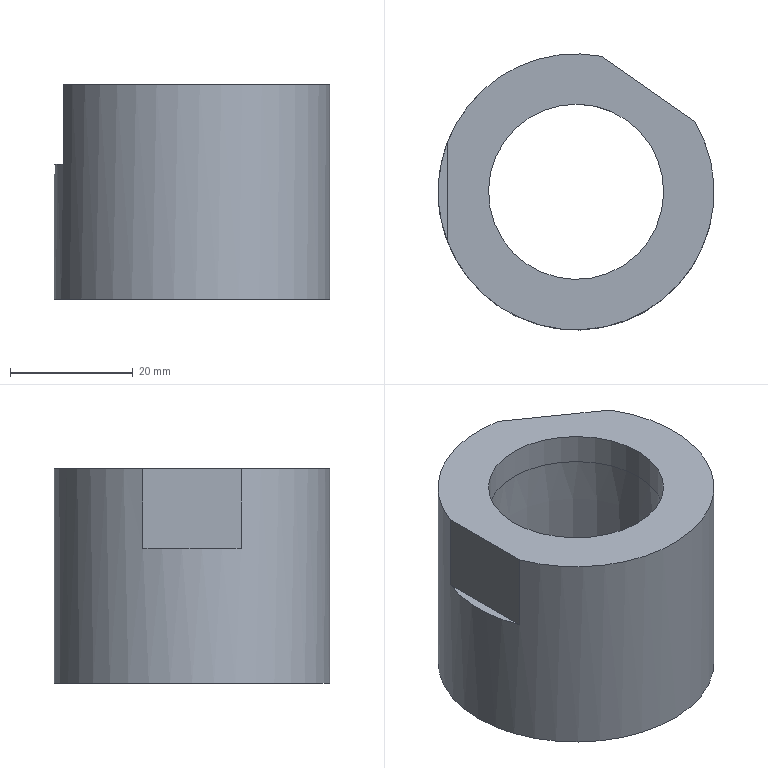Part | STEP file | lll_id4538_x_t | 1 solid | 10 faces | box 45 x 45 x 35 mm | volume 31065 mm3 | plane 7 | cylinder 2 | cone 1 | commonest cylinder face diameters 28.57 x1 45 x1
STEP:
#1=CARTESIAN_POINT('',(3349.528,65.399,-35.));
#2=VERTEX_POINT('',#1);
#3=CARTESIAN_POINT('',(3364.721,54.761,-35.));
#4=VERTEX_POINT('',#3);
#5=CARTESIAN_POINT('',(3361.63,56.926,-35.));
#6=DIRECTION('',(0.8192,-0.5736,0.));
#7=VECTOR('',#6,1.);
#8=LINE('',#5,#7);
#9=EDGE_CURVE('',#2,#4,#8,.T.);
#10=ORIENTED_EDGE('',*,*,#9,.T.);
#11=CARTESIAN_POINT('',(3345.367,43.288,-35.));
#12=DIRECTION('',(0.,0.,-1.));
#13=DIRECTION('',(-1.,0.,0.));
#14=AXIS2_PLACEMENT_3D('',#11,#12,#13);
#15=CIRCLE('',#14,22.5);
#16=EDGE_CURVE('',#4,#2,#15,.T.);
#17=ORIENTED_EDGE('',*,*,#16,.T.);
#18=EDGE_LOOP('',(#10,#17));
#19=FACE_BOUND('',#18,.T.);
#20=CARTESIAN_POINT('',(3330.296,43.288,-35.));
#21=VERTEX_POINT('',#20);
#22=CARTESIAN_POINT('',(3345.367,43.288,-35.));
#23=DIRECTION('',(0.,0.,1.));
#24=DIRECTION('',(-1.,0.,0.));
#25=AXIS2_PLACEMENT_3D('',#22,#23,#24);
#26=CIRCLE('',#25,15.071);
#27=EDGE_CURVE('',#21,#21,#26,.T.);
#28=ORIENTED_EDGE('',*,*,#27,.T.);
#29=EDGE_LOOP('',(#28));
#30=FACE_BOUND('',#29,.T.);
#31=CARTESIAN_POINT('',(3349.872,40.133,-35.));
#32=DIRECTION('',(0.,0.,-1.));
#33=DIRECTION('',(-0.8192,0.5736,0.));
#34=AXIS2_PLACEMENT_3D('',#31,#32,#33);
#35=PLANE('',#34);
#36=ADVANCED_FACE('',(#19,#30),#35,.T.);
#37=CARTESIAN_POINT('',(3337.173,31.586,0.00001711));
#38=VERTEX_POINT('',#37);
#39=CARTESIAN_POINT('',(3345.367,43.288,0.00001711));
#40=DIRECTION('',(0.,0.,-1.));
#41=DIRECTION('',(-0.5736,-0.8192,0.));
#42=AXIS2_PLACEMENT_3D('',#39,#40,#41);
#43=CIRCLE('',#42,14.285);
#44=EDGE_CURVE('',#38,#38,#43,.T.);
#45=ORIENTED_EDGE('',*,*,#44,.F.);
#46=EDGE_LOOP('',(#45));
#47=FACE_BOUND('',#46,.T.);
#48=CARTESIAN_POINT('',(3337.173,31.586,-5.));
#49=VERTEX_POINT('',#48);
#50=CARTESIAN_POINT('',(3345.367,43.288,-5.));
#51=DIRECTION('',(0.,0.,-1.));
#52=DIRECTION('',(-0.5736,-0.8192,0.));
#53=AXIS2_PLACEMENT_3D('',#50,#51,#52);
#54=CIRCLE('',#53,14.285);
#55=EDGE_CURVE('',#49,#49,#54,.T.);
#56=ORIENTED_EDGE('',*,*,#55,.T.);
#57=EDGE_LOOP('',(#56));
#58=FACE_BOUND('',#57,.T.);
#59=CARTESIAN_POINT('',(3345.367,43.288,-2.4));
#60=DIRECTION('',(0.,0.,1.));
#61=DIRECTION('',(-0.5736,-0.8192,0.));
#62=AXIS2_PLACEMENT_3D('',#59,#60,#61);
#63=CYLINDRICAL_SURFACE('',#62,14.285);
#64=ADVANCED_FACE('',(#47,#58),#63,.F.);
#65=CARTESIAN_POINT('',(3364.721,54.761,0.00001711));
#66=VERTEX_POINT('',#65);
#67=CARTESIAN_POINT('',(3324.337,35.288,0.00001711));
#68=VERTEX_POINT('',#67);
#69=CARTESIAN_POINT('',(3345.367,43.288,0.00001711));
#70=DIRECTION('',(0.,0.,-1.));
#71=DIRECTION('',(-0.5736,-0.8192,0.));
#72=AXIS2_PLACEMENT_3D('',#69,#70,#71);
#73=CIRCLE('',#72,22.5);
#74=EDGE_CURVE('',#66,#68,#73,.T.);
#75=ORIENTED_EDGE('',*,*,#74,.T.);
#76=CARTESIAN_POINT('',(3324.337,35.288,-13.));
#77=VERTEX_POINT('',#76);
#78=CARTESIAN_POINT('',(3324.337,35.288,-15.));
#79=DIRECTION('',(0.,0.,1.));
#80=VECTOR('',#79,1.);
#81=LINE('',#78,#80);
#82=EDGE_CURVE('',#77,#68,#81,.T.);
#83=ORIENTED_EDGE('',*,*,#82,.F.);
#84=CARTESIAN_POINT('',(3324.337,51.288,-13.));
#85=VERTEX_POINT('',#84);
#86=CARTESIAN_POINT('',(3345.367,43.288,-13.));
#87=DIRECTION('',(0.,0.,1.));
#88=DIRECTION('',(-1.,0.,0.));
#89=AXIS2_PLACEMENT_3D('',#86,#87,#88);
#90=CIRCLE('',#89,22.5);
#91=EDGE_CURVE('',#85,#77,#90,.T.);
#92=ORIENTED_EDGE('',*,*,#91,.F.);
#93=CARTESIAN_POINT('',(3324.337,51.288,0.00001711));
#94=VERTEX_POINT('',#93);
#95=CARTESIAN_POINT('',(3324.337,51.288,-15.));
#96=DIRECTION('',(0.,0.,-1.));
#97=VECTOR('',#96,1.);
#98=LINE('',#95,#97);
#99=EDGE_CURVE('',#94,#85,#98,.T.);
#100=ORIENTED_EDGE('',*,*,#99,.F.);
#101=CARTESIAN_POINT('',(3349.528,65.399,0.00001711));
#102=VERTEX_POINT('',#101);
#103=CARTESIAN_POINT('',(3345.367,43.288,0.00001711));
#104=DIRECTION('',(0.,0.,-1.));
#105=DIRECTION('',(-0.5736,-0.8192,0.));
#106=AXIS2_PLACEMENT_3D('',#103,#104,#105);
#107=CIRCLE('',#106,22.5);
#108=EDGE_CURVE('',#94,#102,#107,.T.);
#109=ORIENTED_EDGE('',*,*,#108,.T.);
#110=CARTESIAN_POINT('',(3349.528,65.399,-15.));
#111=DIRECTION('',(0.,0.,-1.));
#112=VECTOR('',#111,1.);
#113=LINE('',#110,#112);
#114=EDGE_CURVE('',#102,#2,#113,.T.);
#115=ORIENTED_EDGE('',*,*,#114,.T.);
#116=ORIENTED_EDGE('',*,*,#16,.F.);
#117=CARTESIAN_POINT('',(3364.721,54.761,-15.));
#118=DIRECTION('',(0.,0.,1.));
#119=VECTOR('',#118,1.);
#120=LINE('',#117,#119);
#121=EDGE_CURVE('',#4,#66,#120,.T.);
#122=ORIENTED_EDGE('',*,*,#121,.T.);
#123=EDGE_LOOP('',(#75,#83,#92,#100,#109,#115,#116,#122));
#124=FACE_OUTER_BOUND('',#123,.T.);
#125=CARTESIAN_POINT('',(3345.367,43.288,-15.));
#126=DIRECTION('',(0.,0.,-1.));
#127=DIRECTION('',(0.8192,-0.5736,0.));
#128=AXIS2_PLACEMENT_3D('',#125,#126,#127);
#129=CYLINDRICAL_SURFACE('',#128,22.5);
#130=ADVANCED_FACE('',(#124),#129,.T.);
#131=CARTESIAN_POINT('',(3324.367,35.288,0.00001711));
#132=VERTEX_POINT('',#131);
#133=CARTESIAN_POINT('',(3324.367,51.288,0.00001711));
#134=VERTEX_POINT('',#133);
#135=CARTESIAN_POINT('',(3324.367,43.288,0.00001711));
#136=DIRECTION('',(0.,1.,0.));
#137=VECTOR('',#136,1.);
#138=LINE('',#135,#137);
#139=EDGE_CURVE('',#132,#134,#138,.T.);
#140=ORIENTED_EDGE('',*,*,#139,.F.);
#141=CARTESIAN_POINT('',(3316.367,35.288,0.00001711));
#142=DIRECTION('',(-1.,0.,0.));
#143=VECTOR('',#142,1.);
#144=LINE('',#141,#143);
#145=EDGE_CURVE('',#132,#68,#144,.T.);
#146=ORIENTED_EDGE('',*,*,#145,.T.);
#147=ORIENTED_EDGE('',*,*,#74,.F.);
#148=CARTESIAN_POINT('',(3357.125,60.08,0.00001711));
#149=DIRECTION('',(-0.8192,0.5736,0.));
#150=VECTOR('',#149,1.);
#151=LINE('',#148,#150);
#152=EDGE_CURVE('',#66,#102,#151,.T.);
#153=ORIENTED_EDGE('',*,*,#152,.T.);
#154=ORIENTED_EDGE('',*,*,#108,.F.);
#155=CARTESIAN_POINT('',(3345.367,51.288,0.00001711));
#156=DIRECTION('',(-1.,0.,0.));
#157=VECTOR('',#156,1.);
#158=LINE('',#155,#157);
#159=EDGE_CURVE('',#134,#94,#158,.T.);
#160=ORIENTED_EDGE('',*,*,#159,.F.);
#161=EDGE_LOOP('',(#140,#146,#147,#153,#154,#160));
#162=FACE_BOUND('',#161,.T.);
#163=ORIENTED_EDGE('',*,*,#44,.T.);
#164=EDGE_LOOP('',(#163));
#165=FACE_BOUND('',#164,.T.);
#166=CARTESIAN_POINT('',(3345.367,43.288,0.00001711));
#167=DIRECTION('',(0.,0.,1.));
#168=DIRECTION('',(0.5736,0.8192,0.));
#169=AXIS2_PLACEMENT_3D('',#166,#167,#168);
#170=PLANE('',#169);
#171=ADVANCED_FACE('',(#162,#165),#170,.T.);
#172=ORIENTED_EDGE('',*,*,#9,.F.);
#173=ORIENTED_EDGE('',*,*,#114,.F.);
#174=ORIENTED_EDGE('',*,*,#152,.F.);
#175=ORIENTED_EDGE('',*,*,#121,.F.);
#176=EDGE_LOOP('',(#172,#173,#174,#175));
#177=FACE_OUTER_BOUND('',#176,.T.);
#178=CARTESIAN_POINT('',(3357.125,60.08,-32.5));
#179=DIRECTION('',(0.5736,0.8192,0.));
#180=DIRECTION('',(0.,0.,1.));
#181=AXIS2_PLACEMENT_3D('',#178,#179,#180);
#182=PLANE('',#181);
#183=ADVANCED_FACE('',(#177),#182,.T.);
#184=ORIENTED_EDGE('',*,*,#27,.F.);
#185=EDGE_LOOP('',(#184));
#186=FACE_BOUND('',#185,.T.);
#187=ORIENTED_EDGE('',*,*,#55,.F.);
#188=EDGE_LOOP('',(#187));
#189=FACE_BOUND('',#188,.T.);
#190=CARTESIAN_POINT('',(3345.367,43.288,-5.));
#191=DIRECTION('',(0.,0.,-1.));
#192=DIRECTION('',(-0.5736,-0.8192,0.));
#193=AXIS2_PLACEMENT_3D('',#190,#191,#192);
#194=CONICAL_SURFACE('',#193,14.285,1.5);
#195=ADVANCED_FACE('',(#186,#189),#194,.F.);
#196=ORIENTED_EDGE('',*,*,#145,.F.);
#197=CARTESIAN_POINT('',(3324.367,35.288,-13.));
#198=VERTEX_POINT('',#197);
#199=CARTESIAN_POINT('',(3324.367,35.288,-1.));
#200=DIRECTION('',(0.,0.,-1.));
#201=VECTOR('',#200,1.);
#202=LINE('',#199,#201);
#203=EDGE_CURVE('',#132,#198,#202,.T.);
#204=ORIENTED_EDGE('',*,*,#203,.T.);
#205=CARTESIAN_POINT('',(3316.367,35.288,-13.));
#206=DIRECTION('',(-1.,0.,0.));
#207=VECTOR('',#206,1.);
#208=LINE('',#205,#207);
#209=EDGE_CURVE('',#198,#77,#208,.T.);
#210=ORIENTED_EDGE('',*,*,#209,.T.);
#211=ORIENTED_EDGE('',*,*,#82,.T.);
#212=EDGE_LOOP('',(#196,#204,#210,#211));
#213=FACE_OUTER_BOUND('',#212,.T.);
#214=CARTESIAN_POINT('',(3316.367,35.288,-1.));
#215=DIRECTION('',(0.,-1.,0.));
#216=DIRECTION('',(0.,0.,1.));
#217=AXIS2_PLACEMENT_3D('',#214,#215,#216);
#218=PLANE('',#217);
#219=ADVANCED_FACE('',(#213),#218,.F.);
#220=ORIENTED_EDGE('',*,*,#91,.T.);
#221=ORIENTED_EDGE('',*,*,#209,.F.);
#222=CARTESIAN_POINT('',(3324.367,51.288,-13.));
#223=VERTEX_POINT('',#222);
#224=CARTESIAN_POINT('',(3324.367,43.288,-13.));
#225=DIRECTION('',(0.,-1.,0.));
#226=VECTOR('',#225,1.);
#227=LINE('',#224,#226);
#228=EDGE_CURVE('',#223,#198,#227,.T.);
#229=ORIENTED_EDGE('',*,*,#228,.F.);
#230=CARTESIAN_POINT('',(3316.367,51.288,-13.));
#231=DIRECTION('',(1.,0.,0.));
#232=VECTOR('',#231,1.);
#233=LINE('',#230,#232);
#234=EDGE_CURVE('',#85,#223,#233,.T.);
#235=ORIENTED_EDGE('',*,*,#234,.F.);
#236=EDGE_LOOP('',(#220,#221,#229,#235));
#237=FACE_OUTER_BOUND('',#236,.T.);
#238=CARTESIAN_POINT('',(3316.367,43.288,-13.));
#239=DIRECTION('',(0.,0.,-1.));
#240=DIRECTION('',(1.,0.,0.));
#241=AXIS2_PLACEMENT_3D('',#238,#239,#240);
#242=PLANE('',#241);
#243=ADVANCED_FACE('',(#237),#242,.F.);
#244=CARTESIAN_POINT('',(3324.367,51.288,-1.));
#245=DIRECTION('',(0.,0.,-1.));
#246=VECTOR('',#245,1.);
#247=LINE('',#244,#246);
#248=EDGE_CURVE('',#134,#223,#247,.T.);
#249=ORIENTED_EDGE('',*,*,#248,.F.);
#250=ORIENTED_EDGE('',*,*,#159,.T.);
#251=ORIENTED_EDGE('',*,*,#99,.T.);
#252=ORIENTED_EDGE('',*,*,#234,.T.);
#253=EDGE_LOOP('',(#249,#250,#251,#252));
#254=FACE_OUTER_BOUND('',#253,.T.);
#255=CARTESIAN_POINT('',(3316.367,51.288,-1.));
#256=DIRECTION('',(0.,1.,0.));
#257=DIRECTION('',(0.,0.,-1.));
#258=AXIS2_PLACEMENT_3D('',#255,#256,#257);
#259=PLANE('',#258);
#260=ADVANCED_FACE('',(#254),#259,.F.);
#261=ORIENTED_EDGE('',*,*,#203,.F.);
#262=ORIENTED_EDGE('',*,*,#139,.T.);
#263=ORIENTED_EDGE('',*,*,#248,.T.);
#264=ORIENTED_EDGE('',*,*,#228,.T.);
#265=EDGE_LOOP('',(#261,#262,#263,#264));
#266=FACE_OUTER_BOUND('',#265,.T.);
#267=CARTESIAN_POINT('',(3324.367,43.288,-1.));
#268=DIRECTION('',(1.,0.,0.));
#269=DIRECTION('',(0.,0.,1.));
#270=AXIS2_PLACEMENT_3D('',#267,#268,#269);
#271=PLANE('',#270);
#272=ADVANCED_FACE('',(#266),#271,.F.);
#273=CLOSED_SHELL('',(#36,#64,#130,#171,#183,#195,#219,#243,#260,#272));
#274=MANIFOLD_SOLID_BREP('',#273);
#275=(LENGTH_UNIT()NAMED_UNIT(*)SI_UNIT(.MILLI.,.METRE.));
#276=UNCERTAINTY_MEASURE_WITH_UNIT(LENGTH_MEASURE(0.00002),#275,'','');
#277=(NAMED_UNIT(*)PLANE_ANGLE_UNIT()SI_UNIT($,.RADIAN.));
#278=PLANE_ANGLE_MEASURE_WITH_UNIT(PLANE_ANGLE_MEASURE(0.01745),#277);
#279=DIMENSIONAL_EXPONENTS(0.,0.,0.,0.,0.,0.,0.);
#280=(CONVERSION_BASED_UNIT('DEGREE',#278)NAMED_UNIT(#279)PLANE_ANGLE_UNIT());
#281=(NAMED_UNIT(*)SI_UNIT($,.STERADIAN.)SOLID_ANGLE_UNIT());
#282=(GEOMETRIC_REPRESENTATION_CONTEXT(3)GLOBAL_UNCERTAINTY_ASSIGNED_CONTEXT((#276))GLOBAL_UNIT_ASSIGNED_CONTEXT((#275,#280,#281))REPRESENTATION_CONTEXT('',''));
#283=ADVANCED_BREP_SHAPE_REPRESENTATION('',(#274),#282);